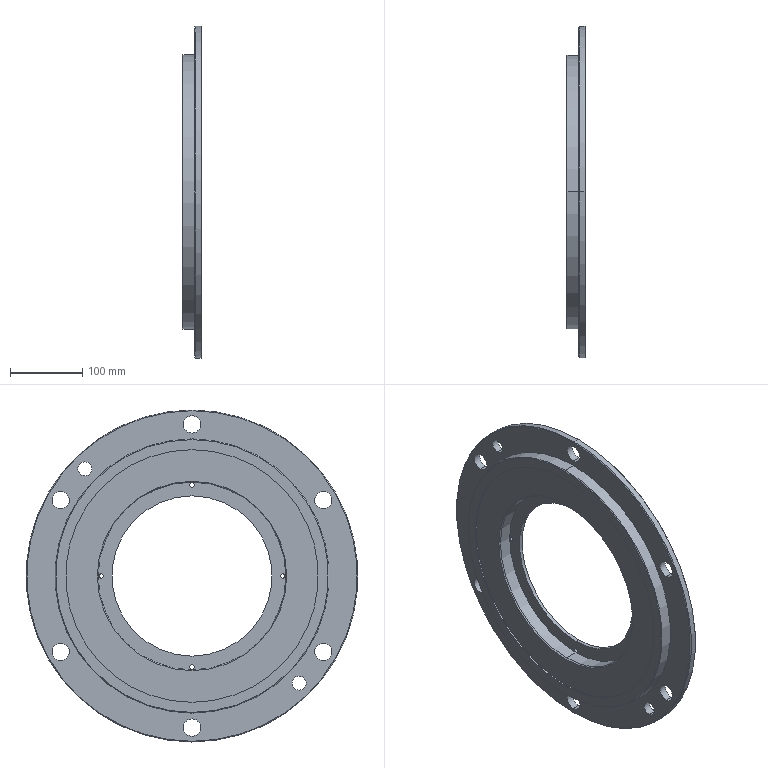Part | SolidWorks | features ICE 4, CirPattern 3, Chamfer 2, 3DProfileFeature 1, HoleWzd 1, Revolution 1 | 1 solid | 47 faces | box 27 x 460 x 460 mm | volume 2105445 mm3 | cylinder 34 | cone 8 | plane 5 | commonest cylinder face diameters 24 x12 6 x8 19.446 x4 222 x2 260 x2 350 x2
STEP:
#1=CARTESIAN_POINT('',(-10.,-148.492,-138.769));
#2=VERTEX_POINT('',#1);
#3=CARTESIAN_POINT('',(-10.,-148.492,-158.216));
#4=VERTEX_POINT('',#3);
#5=CARTESIAN_POINT('',(-10.,-148.492,-148.492));
#6=DIRECTION('',(1.,0.,0.));
#7=DIRECTION('',(0.,0.,-1.));
#8=AXIS2_PLACEMENT_3D('',#5,#6,#7);
#9=CIRCLE('',#8,9.723);
#10=EDGE_CURVE('',#2,#4,#9,.T.);
#11=ORIENTED_EDGE('',*,*,#10,.F.);
#12=CARTESIAN_POINT('',(0.,-148.492,-138.769));
#13=VERTEX_POINT('',#12);
#14=CARTESIAN_POINT('',(0.,-148.492,-138.769));
#15=DIRECTION('',(1.,0.,0.));
#16=VECTOR('',#15,1000.);
#17=LINE('',#14,#16);
#18=EDGE_CURVE('',#2,#13,#17,.T.);
#19=ORIENTED_EDGE('',*,*,#18,.T.);
#20=CARTESIAN_POINT('',(0.,-148.492,-158.216));
#21=VERTEX_POINT('',#20);
#22=CARTESIAN_POINT('',(0.,-148.492,-148.492));
#23=DIRECTION('',(1.,0.,0.));
#24=DIRECTION('',(0.,0.,-1.));
#25=AXIS2_PLACEMENT_3D('',#22,#23,#24);
#26=CIRCLE('',#25,9.723);
#27=EDGE_CURVE('',#13,#21,#26,.T.);
#28=ORIENTED_EDGE('',*,*,#27,.T.);
#29=CARTESIAN_POINT('',(0.,-148.492,-158.216));
#30=DIRECTION('',(1.,0.,0.));
#31=VECTOR('',#30,1000.);
#32=LINE('',#29,#31);
#33=EDGE_CURVE('',#4,#21,#32,.T.);
#34=ORIENTED_EDGE('',*,*,#33,.F.);
#35=EDGE_LOOP('',(#11,#19,#28,#34));
#36=FACE_OUTER_BOUND('',#35,.T.);
#37=CARTESIAN_POINT('',(0.,-148.492,-148.492));
#38=DIRECTION('',(1.,0.,0.));
#39=DIRECTION('',(0.,0.,-1.));
#40=AXIS2_PLACEMENT_3D('',#37,#38,#39);
#41=CYLINDRICAL_SURFACE('',#40,9.723);
#42=ADVANCED_FACE('',(#36),#41,.F.);
#43=CARTESIAN_POINT('',(-10.,148.492,158.216));
#44=VERTEX_POINT('',#43);
#45=CARTESIAN_POINT('',(-10.,148.492,138.769));
#46=VERTEX_POINT('',#45);
#47=CARTESIAN_POINT('',(-10.,148.492,148.492));
#48=DIRECTION('',(1.,0.,0.));
#49=DIRECTION('',(0.,0.,-1.));
#50=AXIS2_PLACEMENT_3D('',#47,#48,#49);
#51=CIRCLE('',#50,9.723);
#52=EDGE_CURVE('',#44,#46,#51,.T.);
#53=ORIENTED_EDGE('',*,*,#52,.F.);
#54=CARTESIAN_POINT('',(0.,148.492,158.216));
#55=VERTEX_POINT('',#54);
#56=CARTESIAN_POINT('',(0.,148.492,158.216));
#57=DIRECTION('',(1.,0.,0.));
#58=VECTOR('',#57,1000.);
#59=LINE('',#56,#58);
#60=EDGE_CURVE('',#44,#55,#59,.T.);
#61=ORIENTED_EDGE('',*,*,#60,.T.);
#62=CARTESIAN_POINT('',(0.,148.492,138.769));
#63=VERTEX_POINT('',#62);
#64=CARTESIAN_POINT('',(0.,148.492,148.492));
#65=DIRECTION('',(1.,0.,0.));
#66=DIRECTION('',(0.,0.,-1.));
#67=AXIS2_PLACEMENT_3D('',#64,#65,#66);
#68=CIRCLE('',#67,9.723);
#69=EDGE_CURVE('',#55,#63,#68,.T.);
#70=ORIENTED_EDGE('',*,*,#69,.T.);
#71=CARTESIAN_POINT('',(0.,148.492,138.769));
#72=DIRECTION('',(1.,0.,0.));
#73=VECTOR('',#72,1000.);
#74=LINE('',#71,#73);
#75=EDGE_CURVE('',#46,#63,#74,.T.);
#76=ORIENTED_EDGE('',*,*,#75,.F.);
#77=EDGE_LOOP('',(#53,#61,#70,#76));
#78=FACE_OUTER_BOUND('',#77,.T.);
#79=CARTESIAN_POINT('',(0.,148.492,148.492));
#80=DIRECTION('',(1.,0.,0.));
#81=DIRECTION('',(0.,0.,-1.));
#82=AXIS2_PLACEMENT_3D('',#79,#80,#81);
#83=CYLINDRICAL_SURFACE('',#82,9.723);
#84=ADVANCED_FACE('',(#78),#83,.F.);
#85=CARTESIAN_POINT('',(-27.,0.,189.));
#86=VERTEX_POINT('',#85);
#87=CARTESIAN_POINT('',(-27.,0.,-189.));
#88=VERTEX_POINT('',#87);
#89=CARTESIAN_POINT('',(-27.,0.,0.));
#90=DIRECTION('',(-1.,0.,0.));
#91=DIRECTION('',(0.,0.,-1.));
#92=AXIS2_PLACEMENT_3D('',#89,#90,#91);
#93=CIRCLE('',#92,189.);
#94=EDGE_CURVE('',#86,#88,#93,.T.);
#95=ORIENTED_EDGE('',*,*,#94,.F.);
#96=CARTESIAN_POINT('',(-26.,0.,190.));
#97=VERTEX_POINT('',#96);
#98=CARTESIAN_POINT('',(-27.,0.,189.));
#99=DIRECTION('',(0.7071,0.,0.7071));
#100=VECTOR('',#99,1000.);
#101=LINE('',#98,#100);
#102=EDGE_CURVE('',#86,#97,#101,.T.);
#103=ORIENTED_EDGE('',*,*,#102,.T.);
#104=CARTESIAN_POINT('',(-26.,0.,-190.));
#105=VERTEX_POINT('',#104);
#106=CARTESIAN_POINT('',(-26.,0.,0.));
#107=DIRECTION('',(1.,0.,0.));
#108=DIRECTION('',(0.,0.,-1.));
#109=AXIS2_PLACEMENT_3D('',#106,#107,#108);
#110=CIRCLE('',#109,190.);
#111=EDGE_CURVE('',#105,#97,#110,.T.);
#112=ORIENTED_EDGE('',*,*,#111,.F.);
#113=CARTESIAN_POINT('',(-27.,0.,-189.));
#114=DIRECTION('',(0.7071,0.,-0.7071));
#115=VECTOR('',#114,1000.);
#116=LINE('',#113,#115);
#117=EDGE_CURVE('',#88,#105,#116,.T.);
#118=ORIENTED_EDGE('',*,*,#117,.F.);
#119=EDGE_LOOP('',(#95,#103,#112,#118));
#120=FACE_OUTER_BOUND('',#119,.T.);
#121=CARTESIAN_POINT('',(-27.,0.,0.));
#122=DIRECTION('',(1.,0.,0.));
#123=DIRECTION('',(0.,0.,-1.));
#124=AXIS2_PLACEMENT_3D('',#121,#122,#123);
#125=CONICAL_SURFACE('',#124,189.,0.7854);
#126=ADVANCED_FACE('',(#120),#125,.T.);
#127=CARTESIAN_POINT('',(-10.,0.,229.));
#128=VERTEX_POINT('',#127);
#129=CARTESIAN_POINT('',(-10.,0.,-229.));
#130=VERTEX_POINT('',#129);
#131=CARTESIAN_POINT('',(-10.,0.,0.));
#132=DIRECTION('',(-1.,0.,0.));
#133=DIRECTION('',(0.,0.,-1.));
#134=AXIS2_PLACEMENT_3D('',#131,#132,#133);
#135=CIRCLE('',#134,229.);
#136=EDGE_CURVE('',#128,#130,#135,.T.);
#137=ORIENTED_EDGE('',*,*,#136,.F.);
#138=CARTESIAN_POINT('',(-9.,0.,230.));
#139=VERTEX_POINT('',#138);
#140=CARTESIAN_POINT('',(-10.,0.,229.));
#141=DIRECTION('',(0.7071,0.,0.7071));
#142=VECTOR('',#141,1000.);
#143=LINE('',#140,#142);
#144=EDGE_CURVE('',#128,#139,#143,.T.);
#145=ORIENTED_EDGE('',*,*,#144,.T.);
#146=CARTESIAN_POINT('',(-9.,0.,-230.));
#147=VERTEX_POINT('',#146);
#148=CARTESIAN_POINT('',(-9.,0.,0.));
#149=DIRECTION('',(1.,0.,0.));
#150=DIRECTION('',(0.,0.,-1.));
#151=AXIS2_PLACEMENT_3D('',#148,#149,#150);
#152=CIRCLE('',#151,230.);
#153=EDGE_CURVE('',#147,#139,#152,.T.);
#154=ORIENTED_EDGE('',*,*,#153,.F.);
#155=CARTESIAN_POINT('',(-10.,0.,-229.));
#156=DIRECTION('',(0.7071,0.,-0.7071));
#157=VECTOR('',#156,1000.);
#158=LINE('',#155,#157);
#159=EDGE_CURVE('',#130,#147,#158,.T.);
#160=ORIENTED_EDGE('',*,*,#159,.F.);
#161=EDGE_LOOP('',(#137,#145,#154,#160));
#162=FACE_OUTER_BOUND('',#161,.T.);
#163=CARTESIAN_POINT('',(-10.,0.,0.));
#164=DIRECTION('',(1.,0.,0.));
#165=DIRECTION('',(0.,0.,-1.));
#166=AXIS2_PLACEMENT_3D('',#163,#164,#165);
#167=CONICAL_SURFACE('',#166,229.,0.7854);
#168=ADVANCED_FACE('',(#162),#167,.T.);
#169=CARTESIAN_POINT('',(0.,0.,-229.));
#170=VERTEX_POINT('',#169);
#171=CARTESIAN_POINT('',(0.,0.,229.));
#172=VERTEX_POINT('',#171);
#173=CARTESIAN_POINT('',(0.,0.,0.));
#174=DIRECTION('',(1.,0.,0.));
#175=DIRECTION('',(0.,0.,1.));
#176=AXIS2_PLACEMENT_3D('',#173,#174,#175);
#177=CIRCLE('',#176,229.);
#178=EDGE_CURVE('',#170,#172,#177,.T.);
#179=ORIENTED_EDGE('',*,*,#178,.F.);
#180=CARTESIAN_POINT('',(-1.,0.,-230.));
#181=VERTEX_POINT('',#180);
#182=CARTESIAN_POINT('',(-1.,0.,-230.));
#183=DIRECTION('',(-0.7071,0.,-0.7071));
#184=VECTOR('',#183,1000.);
#185=LINE('',#182,#184);
#186=EDGE_CURVE('',#170,#181,#185,.T.);
#187=ORIENTED_EDGE('',*,*,#186,.T.);
#188=CARTESIAN_POINT('',(-1.,0.,230.));
#189=VERTEX_POINT('',#188);
#190=CARTESIAN_POINT('',(-1.,0.,0.));
#191=DIRECTION('',(-1.,0.,0.));
#192=DIRECTION('',(0.,0.,1.));
#193=AXIS2_PLACEMENT_3D('',#190,#191,#192);
#194=CIRCLE('',#193,230.);
#195=EDGE_CURVE('',#189,#181,#194,.T.);
#196=ORIENTED_EDGE('',*,*,#195,.F.);
#197=CARTESIAN_POINT('',(-1.,0.,230.));
#198=DIRECTION('',(-0.7071,0.,0.7071));
#199=VECTOR('',#198,1000.);
#200=LINE('',#197,#199);
#201=EDGE_CURVE('',#172,#189,#200,.T.);
#202=ORIENTED_EDGE('',*,*,#201,.F.);
#203=EDGE_LOOP('',(#179,#187,#196,#202));
#204=FACE_OUTER_BOUND('',#203,.T.);
#205=CARTESIAN_POINT('',(-1.,0.,0.));
#206=DIRECTION('',(-1.,0.,0.));
#207=DIRECTION('',(0.,0.,1.));
#208=AXIS2_PLACEMENT_3D('',#205,#206,#207);
#209=CONICAL_SURFACE('',#208,230.,0.7854);
#210=ADVANCED_FACE('',(#204),#209,.T.);
#211=CARTESIAN_POINT('',(-23.,0.,-130.));
#212=VERTEX_POINT('',#211);
#213=CARTESIAN_POINT('',(-23.,0.,130.));
#214=VERTEX_POINT('',#213);
#215=CARTESIAN_POINT('',(-23.,0.,0.));
#216=DIRECTION('',(-1.,0.,0.));
#217=DIRECTION('',(0.,0.,1.));
#218=AXIS2_PLACEMENT_3D('',#215,#216,#217);
#219=CIRCLE('',#218,130.);
#220=EDGE_CURVE('',#212,#214,#219,.T.);
#221=ORIENTED_EDGE('',*,*,#220,.F.);
#222=CARTESIAN_POINT('',(-25.,0.,-131.155));
#223=VERTEX_POINT('',#222);
#224=CARTESIAN_POINT('',(-25.,0.,-131.155));
#225=DIRECTION('',(-0.866,0.,-0.5));
#226=VECTOR('',#225,1000.);
#227=LINE('',#224,#226);
#228=EDGE_CURVE('',#212,#223,#227,.T.);
#229=ORIENTED_EDGE('',*,*,#228,.T.);
#230=CARTESIAN_POINT('',(-25.,0.,131.155));
#231=VERTEX_POINT('',#230);
#232=CARTESIAN_POINT('',(-25.,0.,0.));
#233=DIRECTION('',(1.,0.,0.));
#234=DIRECTION('',(0.,0.,1.));
#235=AXIS2_PLACEMENT_3D('',#232,#233,#234);
#236=CIRCLE('',#235,131.155);
#237=EDGE_CURVE('',#231,#223,#236,.T.);
#238=ORIENTED_EDGE('',*,*,#237,.F.);
#239=CARTESIAN_POINT('',(-25.,0.,131.155));
#240=DIRECTION('',(-0.866,0.,0.5));
#241=VECTOR('',#240,1000.);
#242=LINE('',#239,#241);
#243=EDGE_CURVE('',#214,#231,#242,.T.);
#244=ORIENTED_EDGE('',*,*,#243,.F.);
#245=EDGE_LOOP('',(#221,#229,#238,#244));
#246=FACE_OUTER_BOUND('',#245,.T.);
#247=CARTESIAN_POINT('',(-25.,0.,0.));
#248=DIRECTION('',(-1.,0.,0.));
#249=DIRECTION('',(0.,0.,1.));
#250=AXIS2_PLACEMENT_3D('',#247,#248,#249);
#251=CONICAL_SURFACE('',#250,131.155,0.5236);
#252=ADVANCED_FACE('',(#246),#251,.F.);
#253=CARTESIAN_POINT('',(-25.,0.,-175.));
#254=VERTEX_POINT('',#253);
#255=CARTESIAN_POINT('',(-25.,0.,175.));
#256=VERTEX_POINT('',#255);
#257=CARTESIAN_POINT('',(-25.,0.,0.));
#258=DIRECTION('',(-1.,0.,0.));
#259=DIRECTION('',(0.,0.,1.));
#260=AXIS2_PLACEMENT_3D('',#257,#258,#259);
#261=CIRCLE('',#260,175.);
#262=EDGE_CURVE('',#254,#256,#261,.T.);
#263=ORIENTED_EDGE('',*,*,#262,.F.);
#264=CARTESIAN_POINT('',(-27.,0.,-175.));
#265=VERTEX_POINT('',#264);
#266=CARTESIAN_POINT('',(-25.,0.,-175.));
#267=DIRECTION('',(-1.,0.,0.));
#268=VECTOR('',#267,1000.);
#269=LINE('',#266,#268);
#270=EDGE_CURVE('',#254,#265,#269,.T.);
#271=ORIENTED_EDGE('',*,*,#270,.T.);
#272=CARTESIAN_POINT('',(-27.,0.,175.));
#273=VERTEX_POINT('',#272);
#274=CARTESIAN_POINT('',(-27.,0.,0.));
#275=DIRECTION('',(-1.,0.,0.));
#276=DIRECTION('',(0.,0.,1.));
#277=AXIS2_PLACEMENT_3D('',#274,#275,#276);
#278=CIRCLE('',#277,175.);
#279=EDGE_CURVE('',#265,#273,#278,.T.);
#280=ORIENTED_EDGE('',*,*,#279,.T.);
#281=CARTESIAN_POINT('',(-25.,0.,175.));
#282=DIRECTION('',(-1.,0.,0.));
#283=VECTOR('',#282,1000.);
#284=LINE('',#281,#283);
#285=EDGE_CURVE('',#256,#273,#284,.T.);
#286=ORIENTED_EDGE('',*,*,#285,.F.);
#287=EDGE_LOOP('',(#263,#271,#280,#286));
#288=FACE_OUTER_BOUND('',#287,.T.);
#289=CARTESIAN_POINT('',(-25.,0.,0.));
#290=DIRECTION('',(-1.,0.,0.));
#291=DIRECTION('',(0.,0.,1.));
#292=AXIS2_PLACEMENT_3D('',#289,#290,#291);
#293=CYLINDRICAL_SURFACE('',#292,175.);
#294=ADVANCED_FACE('',(#288),#293,.F.);
#295=CARTESIAN_POINT('',(-10.,-181.865,117.));
#296=VERTEX_POINT('',#295);
#297=CARTESIAN_POINT('',(-10.,-181.865,93.));
#298=VERTEX_POINT('',#297);
#299=CARTESIAN_POINT('',(-10.,-181.865,105.));
#300=DIRECTION('',(1.,0.,0.));
#301=DIRECTION('',(0.,0.,-1.));
#302=AXIS2_PLACEMENT_3D('',#299,#300,#301);
#303=CIRCLE('',#302,12.);
#304=EDGE_CURVE('',#296,#298,#303,.T.);
#305=ORIENTED_EDGE('',*,*,#304,.F.);
#306=CARTESIAN_POINT('',(0.,-181.865,117.));
#307=VERTEX_POINT('',#306);
#308=CARTESIAN_POINT('',(-27.,-181.865,117.));
#309=DIRECTION('',(1.,0.,0.));
#310=VECTOR('',#309,1000.);
#311=LINE('',#308,#310);
#312=EDGE_CURVE('',#296,#307,#311,.T.);
#313=ORIENTED_EDGE('',*,*,#312,.T.);
#314=CARTESIAN_POINT('',(0.,-181.865,93.));
#315=VERTEX_POINT('',#314);
#316=CARTESIAN_POINT('',(0.,-181.865,105.));
#317=DIRECTION('',(1.,0.,0.));
#318=DIRECTION('',(0.,0.866,-0.5));
#319=AXIS2_PLACEMENT_3D('',#316,#317,#318);
#320=CIRCLE('',#319,12.);
#321=EDGE_CURVE('',#307,#315,#320,.T.);
#322=ORIENTED_EDGE('',*,*,#321,.T.);
#323=CARTESIAN_POINT('',(-27.,-181.865,93.));
#324=DIRECTION('',(1.,0.,0.));
#325=VECTOR('',#324,1000.);
#326=LINE('',#323,#325);
#327=EDGE_CURVE('',#298,#315,#326,.T.);
#328=ORIENTED_EDGE('',*,*,#327,.F.);
#329=EDGE_LOOP('',(#305,#313,#322,#328));
#330=FACE_OUTER_BOUND('',#329,.T.);
#331=CARTESIAN_POINT('',(-27.,-181.865,105.));
#332=DIRECTION('',(1.,0.,0.));
#333=DIRECTION('',(0.,0.,-1.));
#334=AXIS2_PLACEMENT_3D('',#331,#332,#333);
#335=CYLINDRICAL_SURFACE('',#334,12.);
#336=ADVANCED_FACE('',(#330),#335,.F.);
#337=CARTESIAN_POINT('',(-10.,-181.865,-93.));
#338=VERTEX_POINT('',#337);
#339=CARTESIAN_POINT('',(-10.,-181.865,-117.));
#340=VERTEX_POINT('',#339);
#341=CARTESIAN_POINT('',(-10.,-181.865,-105.));
#342=DIRECTION('',(1.,0.,0.));
#343=DIRECTION('',(0.,0.,-1.));
#344=AXIS2_PLACEMENT_3D('',#341,#342,#343);
#345=CIRCLE('',#344,12.);
#346=EDGE_CURVE('',#338,#340,#345,.T.);
#347=ORIENTED_EDGE('',*,*,#346,.F.);
#348=CARTESIAN_POINT('',(0.,-181.865,-93.));
#349=VERTEX_POINT('',#348);
#350=CARTESIAN_POINT('',(-27.,-181.865,-93.));
#351=DIRECTION('',(1.,0.,0.));
#352=VECTOR('',#351,1000.);
#353=LINE('',#350,#352);
#354=EDGE_CURVE('',#338,#349,#353,.T.);
#355=ORIENTED_EDGE('',*,*,#354,.T.);
#356=CARTESIAN_POINT('',(0.,-181.865,-117.));
#357=VERTEX_POINT('',#356);
#358=CARTESIAN_POINT('',(0.,-181.865,-105.));
#359=DIRECTION('',(1.,0.,0.));
#360=DIRECTION('',(0.,0.866,0.5));
#361=AXIS2_PLACEMENT_3D('',#358,#359,#360);
#362=CIRCLE('',#361,12.);
#363=EDGE_CURVE('',#349,#357,#362,.T.);
#364=ORIENTED_EDGE('',*,*,#363,.T.);
#365=CARTESIAN_POINT('',(-27.,-181.865,-117.));
#366=DIRECTION('',(1.,0.,0.));
#367=VECTOR('',#366,1000.);
#368=LINE('',#365,#367);
#369=EDGE_CURVE('',#340,#357,#368,.T.);
#370=ORIENTED_EDGE('',*,*,#369,.F.);
#371=EDGE_LOOP('',(#347,#355,#364,#370));
#372=FACE_OUTER_BOUND('',#371,.T.);
#373=CARTESIAN_POINT('',(-27.,-181.865,-105.));
#374=DIRECTION('',(1.,0.,0.));
#375=DIRECTION('',(0.,0.,-1.));
#376=AXIS2_PLACEMENT_3D('',#373,#374,#375);
#377=CYLINDRICAL_SURFACE('',#376,12.);
#378=ADVANCED_FACE('',(#372),#377,.F.);
#379=CARTESIAN_POINT('',(-10.,0.,-198.));
#380=VERTEX_POINT('',#379);
#381=CARTESIAN_POINT('',(-10.,0.,-222.));
#382=VERTEX_POINT('',#381);
#383=CARTESIAN_POINT('',(-10.,0.,-210.));
#384=DIRECTION('',(1.,0.,0.));
#385=DIRECTION('',(0.,0.,-1.));
#386=AXIS2_PLACEMENT_3D('',#383,#384,#385);
#387=CIRCLE('',#386,12.);
#388=EDGE_CURVE('',#380,#382,#387,.T.);
#389=ORIENTED_EDGE('',*,*,#388,.F.);
#390=CARTESIAN_POINT('',(0.,0.,-198.));
#391=VERTEX_POINT('',#390);
#392=CARTESIAN_POINT('',(-27.,0.,-198.));
#393=DIRECTION('',(1.,0.,0.));
#394=VECTOR('',#393,1000.);
#395=LINE('',#392,#394);
#396=EDGE_CURVE('',#380,#391,#395,.T.);
#397=ORIENTED_EDGE('',*,*,#396,.T.);
#398=CARTESIAN_POINT('',(0.,0.,-222.));
#399=VERTEX_POINT('',#398);
#400=CARTESIAN_POINT('',(0.,0.,-210.));
#401=DIRECTION('',(1.,0.,0.));
#402=DIRECTION('',(0.,0.,1.));
#403=AXIS2_PLACEMENT_3D('',#400,#401,#402);
#404=CIRCLE('',#403,12.);
#405=EDGE_CURVE('',#391,#399,#404,.T.);
#406=ORIENTED_EDGE('',*,*,#405,.T.);
#407=CARTESIAN_POINT('',(-27.,0.,-222.));
#408=DIRECTION('',(1.,0.,0.));
#409=VECTOR('',#408,1000.);
#410=LINE('',#407,#409);
#411=EDGE_CURVE('',#382,#399,#410,.T.);
#412=ORIENTED_EDGE('',*,*,#411,.F.);
#413=EDGE_LOOP('',(#389,#397,#406,#412));
#414=FACE_OUTER_BOUND('',#413,.T.);
#415=CARTESIAN_POINT('',(-27.,0.,-210.));
#416=DIRECTION('',(1.,0.,0.));
#417=DIRECTION('',(0.,0.,-1.));
#418=AXIS2_PLACEMENT_3D('',#415,#416,#417);
#419=CYLINDRICAL_SURFACE('',#418,12.);
#420=ADVANCED_FACE('',(#414),#419,.F.);
#421=CARTESIAN_POINT('',(-10.,181.865,-93.));
#422=VERTEX_POINT('',#421);
#423=CARTESIAN_POINT('',(-10.,181.865,-117.));
#424=VERTEX_POINT('',#423);
#425=CARTESIAN_POINT('',(-10.,181.865,-105.));
#426=DIRECTION('',(1.,0.,0.));
#427=DIRECTION('',(0.,0.,-1.));
#428=AXIS2_PLACEMENT_3D('',#425,#426,#427);
#429=CIRCLE('',#428,12.);
#430=EDGE_CURVE('',#422,#424,#429,.T.);
#431=ORIENTED_EDGE('',*,*,#430,.F.);
#432=CARTESIAN_POINT('',(0.,181.865,-93.));
#433=VERTEX_POINT('',#432);
#434=CARTESIAN_POINT('',(-27.,181.865,-93.));
#435=DIRECTION('',(1.,0.,0.));
#436=VECTOR('',#435,1000.);
#437=LINE('',#434,#436);
#438=EDGE_CURVE('',#422,#433,#437,.T.);
#439=ORIENTED_EDGE('',*,*,#438,.T.);
#440=CARTESIAN_POINT('',(0.,181.865,-117.));
#441=VERTEX_POINT('',#440);
#442=CARTESIAN_POINT('',(0.,181.865,-105.));
#443=DIRECTION('',(1.,0.,0.));
#444=DIRECTION('',(0.,-0.866,0.5));
#445=AXIS2_PLACEMENT_3D('',#442,#443,#444);
#446=CIRCLE('',#445,12.);
#447=EDGE_CURVE('',#433,#441,#446,.T.);
#448=ORIENTED_EDGE('',*,*,#447,.T.);
#449=CARTESIAN_POINT('',(-27.,181.865,-117.));
#450=DIRECTION('',(1.,0.,0.));
#451=VECTOR('',#450,1000.);
#452=LINE('',#449,#451);
#453=EDGE_CURVE('',#424,#441,#452,.T.);
#454=ORIENTED_EDGE('',*,*,#453,.F.);
#455=EDGE_LOOP('',(#431,#439,#448,#454));
#456=FACE_OUTER_BOUND('',#455,.T.);
#457=CARTESIAN_POINT('',(-27.,181.865,-105.));
#458=DIRECTION('',(1.,0.,0.));
#459=DIRECTION('',(0.,0.,-1.));
#460=AXIS2_PLACEMENT_3D('',#457,#458,#459);
#461=CYLINDRICAL_SURFACE('',#460,12.);
#462=ADVANCED_FACE('',(#456),#461,.F.);
#463=CARTESIAN_POINT('',(-10.,181.865,117.));
#464=VERTEX_POINT('',#463);
#465=CARTESIAN_POINT('',(-10.,181.865,93.));
#466=VERTEX_POINT('',#465);
#467=CARTESIAN_POINT('',(-10.,181.865,105.));
#468=DIRECTION('',(1.,0.,0.));
#469=DIRECTION('',(0.,0.,-1.));
#470=AXIS2_PLACEMENT_3D('',#467,#468,#469);
#471=CIRCLE('',#470,12.);
#472=EDGE_CURVE('',#464,#466,#471,.T.);
#473=ORIENTED_EDGE('',*,*,#472,.F.);
#474=CARTESIAN_POINT('',(0.,181.865,117.));
#475=VERTEX_POINT('',#474);
#476=CARTESIAN_POINT('',(-27.,181.865,117.));
#477=DIRECTION('',(1.,0.,0.));
#478=VECTOR('',#477,1000.);
#479=LINE('',#476,#478);
#480=EDGE_CURVE('',#464,#475,#479,.T.);
#481=ORIENTED_EDGE('',*,*,#480,.T.);
#482=CARTESIAN_POINT('',(0.,181.865,93.));
#483=VERTEX_POINT('',#482);
#484=CARTESIAN_POINT('',(0.,181.865,105.));
#485=DIRECTION('',(1.,0.,0.));
#486=DIRECTION('',(0.,-0.866,-0.5));
#487=AXIS2_PLACEMENT_3D('',#484,#485,#486);
#488=CIRCLE('',#487,12.);
#489=EDGE_CURVE('',#475,#483,#488,.T.);
#490=ORIENTED_EDGE('',*,*,#489,.T.);
#491=CARTESIAN_POINT('',(-27.,181.865,93.));
#492=DIRECTION('',(1.,0.,0.));
#493=VECTOR('',#492,1000.);
#494=LINE('',#491,#493);
#495=EDGE_CURVE('',#466,#483,#494,.T.);
#496=ORIENTED_EDGE('',*,*,#495,.F.);
#497=EDGE_LOOP('',(#473,#481,#490,#496));
#498=FACE_OUTER_BOUND('',#497,.T.);
#499=CARTESIAN_POINT('',(-27.,181.865,105.));
#500=DIRECTION('',(1.,0.,0.));
#501=DIRECTION('',(0.,0.,-1.));
#502=AXIS2_PLACEMENT_3D('',#499,#500,#501);
#503=CYLINDRICAL_SURFACE('',#502,12.);
#504=ADVANCED_FACE('',(#498),#503,.F.);
#505=CARTESIAN_POINT('',(-10.,0.,222.));
#506=VERTEX_POINT('',#505);
#507=CARTESIAN_POINT('',(-10.,0.,198.));
#508=VERTEX_POINT('',#507);
#509=CARTESIAN_POINT('',(-10.,0.,210.));
#510=DIRECTION('',(1.,0.,0.));
#511=DIRECTION('',(0.,0.,-1.));
#512=AXIS2_PLACEMENT_3D('',#509,#510,#511);
#513=CIRCLE('',#512,12.);
#514=EDGE_CURVE('',#506,#508,#513,.T.);
#515=ORIENTED_EDGE('',*,*,#514,.F.);
#516=CARTESIAN_POINT('',(0.,0.,222.));
#517=VERTEX_POINT('',#516);
#518=CARTESIAN_POINT('',(-27.,0.,222.));
#519=DIRECTION('',(1.,0.,0.));
#520=VECTOR('',#519,1000.);
#521=LINE('',#518,#520);
#522=EDGE_CURVE('',#506,#517,#521,.T.);
#523=ORIENTED_EDGE('',*,*,#522,.T.);
#524=CARTESIAN_POINT('',(0.,0.,198.));
#525=VERTEX_POINT('',#524);
#526=CARTESIAN_POINT('',(0.,0.,210.));
#527=DIRECTION('',(1.,0.,0.));
#528=DIRECTION('',(0.,0.,-1.));
#529=AXIS2_PLACEMENT_3D('',#526,#527,#528);
#530=CIRCLE('',#529,12.);
#531=EDGE_CURVE('',#517,#525,#530,.T.);
#532=ORIENTED_EDGE('',*,*,#531,.T.);
#533=CARTESIAN_POINT('',(-27.,0.,198.));
#534=DIRECTION('',(1.,0.,0.));
#535=VECTOR('',#534,1000.);
#536=LINE('',#533,#535);
#537=EDGE_CURVE('',#508,#525,#536,.T.);
#538=ORIENTED_EDGE('',*,*,#537,.F.);
#539=EDGE_LOOP('',(#515,#523,#532,#538));
#540=FACE_OUTER_BOUND('',#539,.T.);
#541=CARTESIAN_POINT('',(-27.,0.,210.));
#542=DIRECTION('',(1.,0.,0.));
#543=DIRECTION('',(0.,0.,-1.));
#544=AXIS2_PLACEMENT_3D('',#541,#542,#543);
#545=CYLINDRICAL_SURFACE('',#544,12.);
#546=ADVANCED_FACE('',(#540),#545,.F.);
#547=CARTESIAN_POINT('',(-10.,0.,190.));
#548=VERTEX_POINT('',#547);
#549=CARTESIAN_POINT('',(-10.,0.,-190.));
#550=VERTEX_POINT('',#549);
#551=CARTESIAN_POINT('',(-10.,0.,0.));
#552=DIRECTION('',(-1.,0.,0.));
#553=DIRECTION('',(0.,0.,1.));
#554=AXIS2_PLACEMENT_3D('',#551,#552,#553);
#555=CIRCLE('',#554,190.);
#556=EDGE_CURVE('',#548,#550,#555,.T.);
#557=ORIENTED_EDGE('',*,*,#556,.T.);
#558=CARTESIAN_POINT('',(-73.563,0.,-190.));
#559=DIRECTION('',(-1.,0.,0.));
#560=VECTOR('',#559,1000.);
#561=LINE('',#558,#560);
#562=EDGE_CURVE('',#550,#105,#561,.T.);
#563=ORIENTED_EDGE('',*,*,#562,.T.);
#564=ORIENTED_EDGE('',*,*,#111,.T.);
#565=CARTESIAN_POINT('',(-73.563,0.,190.));
#566=DIRECTION('',(-1.,0.,0.));
#567=VECTOR('',#566,1000.);
#568=LINE('',#565,#567);
#569=EDGE_CURVE('',#548,#97,#568,.T.);
#570=ORIENTED_EDGE('',*,*,#569,.F.);
#571=EDGE_LOOP('',(#557,#563,#564,#570));
#572=FACE_OUTER_BOUND('',#571,.T.);
#573=CARTESIAN_POINT('',(-73.563,0.,0.));
#574=DIRECTION('',(-1.,0.,0.));
#575=DIRECTION('',(0.,0.,1.));
#576=AXIS2_PLACEMENT_3D('',#573,#574,#575);
#577=CYLINDRICAL_SURFACE('',#576,190.);
#578=ADVANCED_FACE('',(#572),#577,.T.);
#579=ORIENTED_EDGE('',*,*,#195,.T.);
#580=CARTESIAN_POINT('',(-73.563,0.,-230.));
#581=DIRECTION('',(-1.,0.,0.));
#582=VECTOR('',#581,1000.);
#583=LINE('',#580,#582);
#584=EDGE_CURVE('',#181,#147,#583,.T.);
#585=ORIENTED_EDGE('',*,*,#584,.T.);
#586=ORIENTED_EDGE('',*,*,#153,.T.);
#587=CARTESIAN_POINT('',(-73.563,0.,230.));
#588=DIRECTION('',(-1.,0.,0.));
#589=VECTOR('',#588,1000.);
#590=LINE('',#587,#589);
#591=EDGE_CURVE('',#189,#139,#590,.T.);
#592=ORIENTED_EDGE('',*,*,#591,.F.);
#593=EDGE_LOOP('',(#579,#585,#586,#592));
#594=FACE_OUTER_BOUND('',#593,.T.);
#595=CARTESIAN_POINT('',(-73.563,0.,0.));
#596=DIRECTION('',(-1.,0.,0.));
#597=DIRECTION('',(0.,0.,1.));
#598=AXIS2_PLACEMENT_3D('',#595,#596,#597);
#599=CYLINDRICAL_SURFACE('',#598,230.);
#600=ADVANCED_FACE('',(#594),#599,.T.);
#601=CARTESIAN_POINT('',(-5.,-126.,3.));
#602=VERTEX_POINT('',#601);
#603=CARTESIAN_POINT('',(-5.,-126.,-3.));
#604=VERTEX_POINT('',#603);
#605=CARTESIAN_POINT('',(-5.,-126.,0.));
#606=DIRECTION('',(1.,0.,0.));
#607=DIRECTION('',(0.,0.,1.));
#608=AXIS2_PLACEMENT_3D('',#605,#606,#607);
#609=CIRCLE('',#608,3.);
#610=EDGE_CURVE('',#602,#604,#609,.T.);
#611=ORIENTED_EDGE('',*,*,#610,.F.);
#612=CARTESIAN_POINT('',(0.,-126.,3.));
#613=VERTEX_POINT('',#612);
#614=CARTESIAN_POINT('',(-27.,-126.,3.));
#615=DIRECTION('',(1.,0.,0.));
#616=VECTOR('',#615,1000.);
#617=LINE('',#614,#616);
#618=EDGE_CURVE('',#602,#613,#617,.T.);
#619=ORIENTED_EDGE('',*,*,#618,.T.);
#620=CARTESIAN_POINT('',(0.,-126.,-3.));
#621=VERTEX_POINT('',#620);
#622=CARTESIAN_POINT('',(0.,-126.,0.));
#623=DIRECTION('',(1.,0.,0.));
#624=DIRECTION('',(0.,1.,0.));
#625=AXIS2_PLACEMENT_3D('',#622,#623,#624);
#626=CIRCLE('',#625,3.);
#627=EDGE_CURVE('',#613,#621,#626,.T.);
#628=ORIENTED_EDGE('',*,*,#627,.T.);
#629=CARTESIAN_POINT('',(-27.,-126.,-3.));
#630=DIRECTION('',(1.,0.,0.));
#631=VECTOR('',#630,1000.);
#632=LINE('',#629,#631);
#633=EDGE_CURVE('',#604,#621,#632,.T.);
#634=ORIENTED_EDGE('',*,*,#633,.F.);
#635=EDGE_LOOP('',(#611,#619,#628,#634));
#636=FACE_OUTER_BOUND('',#635,.T.);
#637=CARTESIAN_POINT('',(-27.,-126.,0.));
#638=DIRECTION('',(1.,0.,0.));
#639=DIRECTION('',(0.,0.,-1.));
#640=AXIS2_PLACEMENT_3D('',#637,#638,#639);
#641=CYLINDRICAL_SURFACE('',#640,3.);
#642=ADVANCED_FACE('',(#636),#641,.F.);
#643=CARTESIAN_POINT('',(-5.,0.,-123.));
#644=VERTEX_POINT('',#643);
#645=CARTESIAN_POINT('',(-5.,0.,-129.));
#646=VERTEX_POINT('',#645);
#647=CARTESIAN_POINT('',(-5.,0.,-126.));
#648=DIRECTION('',(1.,0.,0.));
#649=DIRECTION('',(0.,0.,1.));
#650=AXIS2_PLACEMENT_3D('',#647,#648,#649);
#651=CIRCLE('',#650,3.);
#652=EDGE_CURVE('',#644,#646,#651,.T.);
#653=ORIENTED_EDGE('',*,*,#652,.F.);
#654=CARTESIAN_POINT('',(0.,0.,-123.));
#655=VERTEX_POINT('',#654);
#656=CARTESIAN_POINT('',(-27.,0.,-123.));
#657=DIRECTION('',(1.,0.,0.));
#658=VECTOR('',#657,1000.);
#659=LINE('',#656,#658);
#660=EDGE_CURVE('',#644,#655,#659,.T.);
#661=ORIENTED_EDGE('',*,*,#660,.T.);
#662=CARTESIAN_POINT('',(0.,0.,-129.));
#663=VERTEX_POINT('',#662);
#664=CARTESIAN_POINT('',(0.,0.,-126.));
#665=DIRECTION('',(1.,0.,0.));
#666=DIRECTION('',(0.,0.,1.));
#667=AXIS2_PLACEMENT_3D('',#664,#665,#666);
#668=CIRCLE('',#667,3.);
#669=EDGE_CURVE('',#655,#663,#668,.T.);
#670=ORIENTED_EDGE('',*,*,#669,.T.);
#671=CARTESIAN_POINT('',(-27.,0.,-129.));
#672=DIRECTION('',(1.,0.,0.));
#673=VECTOR('',#672,1000.);
#674=LINE('',#671,#673);
#675=EDGE_CURVE('',#646,#663,#674,.T.);
#676=ORIENTED_EDGE('',*,*,#675,.F.);
#677=EDGE_LOOP('',(#653,#661,#670,#676));
#678=FACE_OUTER_BOUND('',#677,.T.);
#679=CARTESIAN_POINT('',(-27.,0.,-126.));
#680=DIRECTION('',(1.,0.,0.));
#681=DIRECTION('',(0.,0.,-1.));
#682=AXIS2_PLACEMENT_3D('',#679,#680,#681);
#683=CYLINDRICAL_SURFACE('',#682,3.);
#684=ADVANCED_FACE('',(#678),#683,.F.);
#685=CARTESIAN_POINT('',(-5.,126.,3.));
#686=VERTEX_POINT('',#685);
#687=CARTESIAN_POINT('',(-5.,126.,-3.));
#688=VERTEX_POINT('',#687);
#689=CARTESIAN_POINT('',(-5.,126.,0.));
#690=DIRECTION('',(1.,0.,0.));
#691=DIRECTION('',(0.,0.,1.));
#692=AXIS2_PLACEMENT_3D('',#689,#690,#691);
#693=CIRCLE('',#692,3.);
#694=EDGE_CURVE('',#686,#688,#693,.T.);
#695=ORIENTED_EDGE('',*,*,#694,.F.);
#696=CARTESIAN_POINT('',(0.,126.,3.));
#697=VERTEX_POINT('',#696);
#698=CARTESIAN_POINT('',(-27.,126.,3.));
#699=DIRECTION('',(1.,0.,0.));
#700=VECTOR('',#699,1000.);
#701=LINE('',#698,#700);
#702=EDGE_CURVE('',#686,#697,#701,.T.);
#703=ORIENTED_EDGE('',*,*,#702,.T.);
#704=CARTESIAN_POINT('',(0.,126.,-3.));
#705=VERTEX_POINT('',#704);
#706=CARTESIAN_POINT('',(0.,126.,0.));
#707=DIRECTION('',(1.,0.,0.));
#708=DIRECTION('',(0.,-1.,0.));
#709=AXIS2_PLACEMENT_3D('',#706,#707,#708);
#710=CIRCLE('',#709,3.);
#711=EDGE_CURVE('',#697,#705,#710,.T.);
#712=ORIENTED_EDGE('',*,*,#711,.T.);
#713=CARTESIAN_POINT('',(-27.,126.,-3.));
#714=DIRECTION('',(1.,0.,0.));
#715=VECTOR('',#714,1000.);
#716=LINE('',#713,#715);
#717=EDGE_CURVE('',#688,#705,#716,.T.);
#718=ORIENTED_EDGE('',*,*,#717,.F.);
#719=EDGE_LOOP('',(#695,#703,#712,#718));
#720=FACE_OUTER_BOUND('',#719,.T.);
#721=CARTESIAN_POINT('',(-27.,126.,0.));
#722=DIRECTION('',(1.,0.,0.));
#723=DIRECTION('',(0.,0.,-1.));
#724=AXIS2_PLACEMENT_3D('',#721,#722,#723);
#725=CYLINDRICAL_SURFACE('',#724,3.);
#726=ADVANCED_FACE('',(#720),#725,.F.);
#727=CARTESIAN_POINT('',(-5.,0.,129.));
#728=VERTEX_POINT('',#727);
#729=CARTESIAN_POINT('',(-5.,0.,123.));
#730=VERTEX_POINT('',#729);
#731=CARTESIAN_POINT('',(-5.,0.,126.));
#732=DIRECTION('',(1.,0.,0.));
#733=DIRECTION('',(0.,0.,1.));
#734=AXIS2_PLACEMENT_3D('',#731,#732,#733);
#735=CIRCLE('',#734,3.);
#736=EDGE_CURVE('',#728,#730,#735,.T.);
#737=ORIENTED_EDGE('',*,*,#736,.F.);
#738=CARTESIAN_POINT('',(0.,0.,129.));
#739=VERTEX_POINT('',#738);
#740=CARTESIAN_POINT('',(-27.,0.,129.));
#741=DIRECTION('',(1.,0.,0.));
#742=VECTOR('',#741,1000.);
#743=LINE('',#740,#742);
#744=EDGE_CURVE('',#728,#739,#743,.T.);
#745=ORIENTED_EDGE('',*,*,#744,.T.);
#746=CARTESIAN_POINT('',(0.,0.,123.));
#747=VERTEX_POINT('',#746);
#748=CARTESIAN_POINT('',(0.,0.,126.));
#749=DIRECTION('',(1.,0.,0.));
#750=DIRECTION('',(0.,0.,-1.));
#751=AXIS2_PLACEMENT_3D('',#748,#749,#750);
#752=CIRCLE('',#751,3.);
#753=EDGE_CURVE('',#739,#747,#752,.T.);
#754=ORIENTED_EDGE('',*,*,#753,.T.);
#755=CARTESIAN_POINT('',(-27.,0.,123.));
#756=DIRECTION('',(1.,0.,0.));
#757=VECTOR('',#756,1000.);
#758=LINE('',#755,#757);
#759=EDGE_CURVE('',#730,#747,#758,.T.);
#760=ORIENTED_EDGE('',*,*,#759,.F.);
#761=EDGE_LOOP('',(#737,#745,#754,#760));
#762=FACE_OUTER_BOUND('',#761,.T.);
#763=CARTESIAN_POINT('',(-27.,0.,126.));
#764=DIRECTION('',(1.,0.,0.));
#765=DIRECTION('',(0.,0.,-1.));
#766=AXIS2_PLACEMENT_3D('',#763,#764,#765);
#767=CYLINDRICAL_SURFACE('',#766,3.);
#768=ADVANCED_FACE('',(#762),#767,.F.);
#769=CARTESIAN_POINT('',(0.,0.,-111.));
#770=VERTEX_POINT('',#769);
#771=CARTESIAN_POINT('',(0.,0.,111.));
#772=VERTEX_POINT('',#771);
#773=CARTESIAN_POINT('',(0.,0.,0.));
#774=DIRECTION('',(-1.,0.,0.));
#775=DIRECTION('',(0.,0.,1.));
#776=AXIS2_PLACEMENT_3D('',#773,#774,#775);
#777=CIRCLE('',#776,111.);
#778=EDGE_CURVE('',#770,#772,#777,.T.);
#779=ORIENTED_EDGE('',*,*,#778,.F.);
#780=CARTESIAN_POINT('',(-5.,0.,-111.));
#781=VERTEX_POINT('',#780);
#782=CARTESIAN_POINT('',(-73.563,0.,-111.));
#783=DIRECTION('',(-1.,0.,0.));
#784=VECTOR('',#783,1000.);
#785=LINE('',#782,#784);
#786=EDGE_CURVE('',#770,#781,#785,.T.);
#787=ORIENTED_EDGE('',*,*,#786,.T.);
#788=CARTESIAN_POINT('',(-5.,0.,111.));
#789=VERTEX_POINT('',#788);
#790=CARTESIAN_POINT('',(-5.,0.,0.));
#791=DIRECTION('',(1.,0.,0.));
#792=DIRECTION('',(0.,0.,1.));
#793=AXIS2_PLACEMENT_3D('',#790,#791,#792);
#794=CIRCLE('',#793,111.);
#795=EDGE_CURVE('',#789,#781,#794,.T.);
#796=ORIENTED_EDGE('',*,*,#795,.F.);
#797=CARTESIAN_POINT('',(-73.563,0.,111.));
#798=DIRECTION('',(-1.,0.,0.));
#799=VECTOR('',#798,1000.);
#800=LINE('',#797,#799);
#801=EDGE_CURVE('',#772,#789,#800,.T.);
#802=ORIENTED_EDGE('',*,*,#801,.F.);
#803=EDGE_LOOP('',(#779,#787,#796,#802));
#804=FACE_OUTER_BOUND('',#803,.T.);
#805=CARTESIAN_POINT('',(-73.563,0.,0.));
#806=DIRECTION('',(-1.,0.,0.));
#807=DIRECTION('',(0.,0.,1.));
#808=AXIS2_PLACEMENT_3D('',#805,#806,#807);
#809=CYLINDRICAL_SURFACE('',#808,111.);
#810=ADVANCED_FACE('',(#804),#809,.F.);
#811=CARTESIAN_POINT('',(-5.,0.,-130.));
#812=VERTEX_POINT('',#811);
#813=CARTESIAN_POINT('',(-5.,0.,130.));
#814=VERTEX_POINT('',#813);
#815=CARTESIAN_POINT('',(-5.,0.,0.));
#816=DIRECTION('',(-1.,0.,0.));
#817=DIRECTION('',(0.,0.,1.));
#818=AXIS2_PLACEMENT_3D('',#815,#816,#817);
#819=CIRCLE('',#818,130.);
#820=EDGE_CURVE('',#812,#814,#819,.T.);
#821=ORIENTED_EDGE('',*,*,#820,.F.);
#822=CARTESIAN_POINT('',(-5.,0.,-130.));
#823=DIRECTION('',(-1.,0.,0.));
#824=VECTOR('',#823,1000.);
#825=LINE('',#822,#824);
#826=EDGE_CURVE('',#812,#212,#825,.T.);
#827=ORIENTED_EDGE('',*,*,#826,.T.);
#828=ORIENTED_EDGE('',*,*,#220,.T.);
#829=CARTESIAN_POINT('',(-5.,0.,130.));
#830=DIRECTION('',(-1.,0.,0.));
#831=VECTOR('',#830,1000.);
#832=LINE('',#829,#831);
#833=EDGE_CURVE('',#814,#214,#832,.T.);
#834=ORIENTED_EDGE('',*,*,#833,.F.);
#835=EDGE_LOOP('',(#821,#827,#828,#834));
#836=FACE_OUTER_BOUND('',#835,.T.);
#837=CARTESIAN_POINT('',(-5.,0.,0.));
#838=DIRECTION('',(-1.,0.,0.));
#839=DIRECTION('',(0.,0.,1.));
#840=AXIS2_PLACEMENT_3D('',#837,#838,#839);
#841=CYLINDRICAL_SURFACE('',#840,130.);
#842=ADVANCED_FACE('',(#836),#841,.F.);
#843=CARTESIAN_POINT('',(0.,148.492,148.492));
#844=DIRECTION('',(1.,0.,0.));
#845=DIRECTION('',(0.,0.,-1.));
#846=AXIS2_PLACEMENT_3D('',#843,#844,#845);
#847=CIRCLE('',#846,9.723);
#848=EDGE_CURVE('',#63,#55,#847,.T.);
#849=ORIENTED_EDGE('',*,*,#848,.F.);
#850=ORIENTED_EDGE('',*,*,#69,.F.);
#851=EDGE_LOOP('',(#849,#850));
#852=FACE_BOUND('',#851,.T.);
#853=CARTESIAN_POINT('',(0.,0.,0.));
#854=DIRECTION('',(1.,0.,0.));
#855=DIRECTION('',(0.,0.,1.));
#856=AXIS2_PLACEMENT_3D('',#853,#854,#855);
#857=CIRCLE('',#856,229.);
#858=EDGE_CURVE('',#172,#170,#857,.T.);
#859=ORIENTED_EDGE('',*,*,#858,.T.);
#860=ORIENTED_EDGE('',*,*,#178,.T.);
#861=EDGE_LOOP('',(#859,#860));
#862=FACE_OUTER_BOUND('',#861,.T.);
#863=CARTESIAN_POINT('',(0.,-126.,0.));
#864=DIRECTION('',(1.,0.,0.));
#865=DIRECTION('',(0.,1.,0.));
#866=AXIS2_PLACEMENT_3D('',#863,#864,#865);
#867=CIRCLE('',#866,3.);
#868=EDGE_CURVE('',#621,#613,#867,.T.);
#869=ORIENTED_EDGE('',*,*,#868,.F.);
#870=ORIENTED_EDGE('',*,*,#627,.F.);
#871=EDGE_LOOP('',(#869,#870));
#872=FACE_BOUND('',#871,.T.);
#873=CARTESIAN_POINT('',(0.,0.,-126.));
#874=DIRECTION('',(1.,0.,0.));
#875=DIRECTION('',(0.,0.,1.));
#876=AXIS2_PLACEMENT_3D('',#873,#874,#875);
#877=CIRCLE('',#876,3.);
#878=EDGE_CURVE('',#663,#655,#877,.T.);
#879=ORIENTED_EDGE('',*,*,#878,.F.);
#880=ORIENTED_EDGE('',*,*,#669,.F.);
#881=EDGE_LOOP('',(#879,#880));
#882=FACE_BOUND('',#881,.T.);
#883=CARTESIAN_POINT('',(0.,126.,0.));
#884=DIRECTION('',(1.,0.,0.));
#885=DIRECTION('',(0.,-1.,0.));
#886=AXIS2_PLACEMENT_3D('',#883,#884,#885);
#887=CIRCLE('',#886,3.);
#888=EDGE_CURVE('',#705,#697,#887,.T.);
#889=ORIENTED_EDGE('',*,*,#888,.F.);
#890=ORIENTED_EDGE('',*,*,#711,.F.);
#891=EDGE_LOOP('',(#889,#890));
#892=FACE_BOUND('',#891,.T.);
#893=CARTESIAN_POINT('',(0.,0.,126.));
#894=DIRECTION('',(1.,0.,0.));
#895=DIRECTION('',(0.,0.,-1.));
#896=AXIS2_PLACEMENT_3D('',#893,#894,#895);
#897=CIRCLE('',#896,3.);
#898=EDGE_CURVE('',#747,#739,#897,.T.);
#899=ORIENTED_EDGE('',*,*,#898,.F.);
#900=ORIENTED_EDGE('',*,*,#753,.F.);
#901=EDGE_LOOP('',(#899,#900));
#902=FACE_BOUND('',#901,.T.);
#903=CARTESIAN_POINT('',(0.,-181.865,105.));
#904=DIRECTION('',(1.,0.,0.));
#905=DIRECTION('',(0.,0.866,-0.5));
#906=AXIS2_PLACEMENT_3D('',#903,#904,#905);
#907=CIRCLE('',#906,12.);
#908=EDGE_CURVE('',#315,#307,#907,.T.);
#909=ORIENTED_EDGE('',*,*,#908,.F.);
#910=ORIENTED_EDGE('',*,*,#321,.F.);
#911=EDGE_LOOP('',(#909,#910));
#912=FACE_BOUND('',#911,.T.);
#913=CARTESIAN_POINT('',(0.,-181.865,-105.));
#914=DIRECTION('',(1.,0.,0.));
#915=DIRECTION('',(0.,0.866,0.5));
#916=AXIS2_PLACEMENT_3D('',#913,#914,#915);
#917=CIRCLE('',#916,12.);
#918=EDGE_CURVE('',#357,#349,#917,.T.);
#919=ORIENTED_EDGE('',*,*,#918,.F.);
#920=ORIENTED_EDGE('',*,*,#363,.F.);
#921=EDGE_LOOP('',(#919,#920));
#922=FACE_BOUND('',#921,.T.);
#923=CARTESIAN_POINT('',(0.,0.,-210.));
#924=DIRECTION('',(1.,0.,0.));
#925=DIRECTION('',(0.,0.,1.));
#926=AXIS2_PLACEMENT_3D('',#923,#924,#925);
#927=CIRCLE('',#926,12.);
#928=EDGE_CURVE('',#399,#391,#927,.T.);
#929=ORIENTED_EDGE('',*,*,#928,.F.);
#930=ORIENTED_EDGE('',*,*,#405,.F.);
#931=EDGE_LOOP('',(#929,#930));
#932=FACE_BOUND('',#931,.T.);
#933=CARTESIAN_POINT('',(0.,181.865,-105.));
#934=DIRECTION('',(1.,0.,0.));
#935=DIRECTION('',(0.,-0.866,0.5));
#936=AXIS2_PLACEMENT_3D('',#933,#934,#935);
#937=CIRCLE('',#936,12.);
#938=EDGE_CURVE('',#441,#433,#937,.T.);
#939=ORIENTED_EDGE('',*,*,#938,.F.);
#940=ORIENTED_EDGE('',*,*,#447,.F.);
#941=EDGE_LOOP('',(#939,#940));
#942=FACE_BOUND('',#941,.T.);
#943=CARTESIAN_POINT('',(0.,181.865,105.));
#944=DIRECTION('',(1.,0.,0.));
#945=DIRECTION('',(0.,-0.866,-0.5));
#946=AXIS2_PLACEMENT_3D('',#943,#944,#945);
#947=CIRCLE('',#946,12.);
#948=EDGE_CURVE('',#483,#475,#947,.T.);
#949=ORIENTED_EDGE('',*,*,#948,.F.);
#950=ORIENTED_EDGE('',*,*,#489,.F.);
#951=EDGE_LOOP('',(#949,#950));
#952=FACE_BOUND('',#951,.T.);
#953=CARTESIAN_POINT('',(0.,0.,210.));
#954=DIRECTION('',(1.,0.,0.));
#955=DIRECTION('',(0.,0.,-1.));
#956=AXIS2_PLACEMENT_3D('',#953,#954,#955);
#957=CIRCLE('',#956,12.);
#958=EDGE_CURVE('',#525,#517,#957,.T.);
#959=ORIENTED_EDGE('',*,*,#958,.F.);
#960=ORIENTED_EDGE('',*,*,#531,.F.);
#961=EDGE_LOOP('',(#959,#960));
#962=FACE_BOUND('',#961,.T.);
#963=CARTESIAN_POINT('',(0.,0.,0.));
#964=DIRECTION('',(-1.,0.,0.));
#965=DIRECTION('',(0.,0.,1.));
#966=AXIS2_PLACEMENT_3D('',#963,#964,#965);
#967=CIRCLE('',#966,111.);
#968=EDGE_CURVE('',#772,#770,#967,.T.);
#969=ORIENTED_EDGE('',*,*,#968,.T.);
#970=ORIENTED_EDGE('',*,*,#778,.T.);
#971=EDGE_LOOP('',(#969,#970));
#972=FACE_BOUND('',#971,.T.);
#973=CARTESIAN_POINT('',(0.,-148.492,-148.492));
#974=DIRECTION('',(1.,0.,0.));
#975=DIRECTION('',(0.,0.,-1.));
#976=AXIS2_PLACEMENT_3D('',#973,#974,#975);
#977=CIRCLE('',#976,9.723);
#978=EDGE_CURVE('',#21,#13,#977,.T.);
#979=ORIENTED_EDGE('',*,*,#978,.F.);
#980=ORIENTED_EDGE('',*,*,#27,.F.);
#981=EDGE_LOOP('',(#979,#980));
#982=FACE_BOUND('',#981,.T.);
#983=CARTESIAN_POINT('',(0.,111.,0.));
#984=DIRECTION('',(-1.,0.,0.));
#985=DIRECTION('',(0.,0.,1.));
#986=AXIS2_PLACEMENT_3D('',#983,#984,#985);
#987=PLANE('',#986);
#988=ADVANCED_FACE('',(#852,#862,#872,#882,#892,#902,#912,#922,#932,#942,#952,#962,#972,#982),#987,.F.);
#989=ORIENTED_EDGE('',*,*,#826,.F.);
#990=CARTESIAN_POINT('',(-5.,0.,0.));
#991=DIRECTION('',(-1.,0.,0.));
#992=DIRECTION('',(0.,0.,1.));
#993=AXIS2_PLACEMENT_3D('',#990,#991,#992);
#994=CIRCLE('',#993,130.);
#995=EDGE_CURVE('',#814,#812,#994,.T.);
#996=ORIENTED_EDGE('',*,*,#995,.F.);
#997=ORIENTED_EDGE('',*,*,#833,.T.);
#998=CARTESIAN_POINT('',(-23.,0.,0.));
#999=DIRECTION('',(-1.,0.,0.));
#1000=DIRECTION('',(0.,0.,1.));
#1001=AXIS2_PLACEMENT_3D('',#998,#999,#1000);
#1002=CIRCLE('',#1001,130.);
#1003=EDGE_CURVE('',#214,#212,#1002,.T.);
#1004=ORIENTED_EDGE('',*,*,#1003,.T.);
#1005=EDGE_LOOP('',(#989,#996,#997,#1004));
#1006=FACE_OUTER_BOUND('',#1005,.T.);
#1007=CARTESIAN_POINT('',(-5.,0.,0.));
#1008=DIRECTION('',(-1.,0.,0.));
#1009=DIRECTION('',(0.,0.,1.));
#1010=AXIS2_PLACEMENT_3D('',#1007,#1008,#1009);
#1011=CYLINDRICAL_SURFACE('',#1010,130.);
#1012=ADVANCED_FACE('',(#1006),#1011,.F.);
#1013=ORIENTED_EDGE('',*,*,#786,.F.);
#1014=ORIENTED_EDGE('',*,*,#968,.F.);
#1015=ORIENTED_EDGE('',*,*,#801,.T.);
#1016=CARTESIAN_POINT('',(-5.,0.,0.));
#1017=DIRECTION('',(1.,0.,0.));
#1018=DIRECTION('',(0.,0.,1.));
#1019=AXIS2_PLACEMENT_3D('',#1016,#1017,#1018);
#1020=CIRCLE('',#1019,111.);
#1021=EDGE_CURVE('',#781,#789,#1020,.T.);
#1022=ORIENTED_EDGE('',*,*,#1021,.F.);
#1023=EDGE_LOOP('',(#1013,#1014,#1015,#1022));
#1024=FACE_OUTER_BOUND('',#1023,.T.);
#1025=CARTESIAN_POINT('',(-73.563,0.,0.));
#1026=DIRECTION('',(-1.,0.,0.));
#1027=DIRECTION('',(0.,0.,1.));
#1028=AXIS2_PLACEMENT_3D('',#1025,#1026,#1027);
#1029=CYLINDRICAL_SURFACE('',#1028,111.);
#1030=ADVANCED_FACE('',(#1024),#1029,.F.);
#1031=ORIENTED_EDGE('',*,*,#744,.F.);
#1032=CARTESIAN_POINT('',(-5.,0.,126.));
#1033=DIRECTION('',(1.,0.,0.));
#1034=DIRECTION('',(0.,0.,1.));
#1035=AXIS2_PLACEMENT_3D('',#1032,#1033,#1034);
#1036=CIRCLE('',#1035,3.);
#1037=EDGE_CURVE('',#730,#728,#1036,.T.);
#1038=ORIENTED_EDGE('',*,*,#1037,.F.);
#1039=ORIENTED_EDGE('',*,*,#759,.T.);
#1040=ORIENTED_EDGE('',*,*,#898,.T.);
#1041=EDGE_LOOP('',(#1031,#1038,#1039,#1040));
#1042=FACE_OUTER_BOUND('',#1041,.T.);
#1043=CARTESIAN_POINT('',(-27.,0.,126.));
#1044=DIRECTION('',(1.,0.,0.));
#1045=DIRECTION('',(0.,0.,-1.));
#1046=AXIS2_PLACEMENT_3D('',#1043,#1044,#1045);
#1047=CYLINDRICAL_SURFACE('',#1046,3.);
#1048=ADVANCED_FACE('',(#1042),#1047,.F.);
#1049=ORIENTED_EDGE('',*,*,#702,.F.);
#1050=CARTESIAN_POINT('',(-5.,126.,0.));
#1051=DIRECTION('',(1.,0.,0.));
#1052=DIRECTION('',(0.,0.,1.));
#1053=AXIS2_PLACEMENT_3D('',#1050,#1051,#1052);
#1054=CIRCLE('',#1053,3.);
#1055=EDGE_CURVE('',#688,#686,#1054,.T.);
#1056=ORIENTED_EDGE('',*,*,#1055,.F.);
#1057=ORIENTED_EDGE('',*,*,#717,.T.);
#1058=ORIENTED_EDGE('',*,*,#888,.T.);
#1059=EDGE_LOOP('',(#1049,#1056,#1057,#1058));
#1060=FACE_OUTER_BOUND('',#1059,.T.);
#1061=CARTESIAN_POINT('',(-27.,126.,0.));
#1062=DIRECTION('',(1.,0.,0.));
#1063=DIRECTION('',(0.,0.,-1.));
#1064=AXIS2_PLACEMENT_3D('',#1061,#1062,#1063);
#1065=CYLINDRICAL_SURFACE('',#1064,3.);
#1066=ADVANCED_FACE('',(#1060),#1065,.F.);
#1067=ORIENTED_EDGE('',*,*,#660,.F.);
#1068=CARTESIAN_POINT('',(-5.,0.,-126.));
#1069=DIRECTION('',(1.,0.,0.));
#1070=DIRECTION('',(0.,0.,1.));
#1071=AXIS2_PLACEMENT_3D('',#1068,#1069,#1070);
#1072=CIRCLE('',#1071,3.);
#1073=EDGE_CURVE('',#646,#644,#1072,.T.);
#1074=ORIENTED_EDGE('',*,*,#1073,.F.);
#1075=ORIENTED_EDGE('',*,*,#675,.T.);
#1076=ORIENTED_EDGE('',*,*,#878,.T.);
#1077=EDGE_LOOP('',(#1067,#1074,#1075,#1076));
#1078=FACE_OUTER_BOUND('',#1077,.T.);
#1079=CARTESIAN_POINT('',(-27.,0.,-126.));
#1080=DIRECTION('',(1.,0.,0.));
#1081=DIRECTION('',(0.,0.,-1.));
#1082=AXIS2_PLACEMENT_3D('',#1079,#1080,#1081);
#1083=CYLINDRICAL_SURFACE('',#1082,3.);
#1084=ADVANCED_FACE('',(#1078),#1083,.F.);
#1085=ORIENTED_EDGE('',*,*,#618,.F.);
#1086=CARTESIAN_POINT('',(-5.,-126.,0.));
#1087=DIRECTION('',(1.,0.,0.));
#1088=DIRECTION('',(0.,0.,1.));
#1089=AXIS2_PLACEMENT_3D('',#1086,#1087,#1088);
#1090=CIRCLE('',#1089,3.);
#1091=EDGE_CURVE('',#604,#602,#1090,.T.);
#1092=ORIENTED_EDGE('',*,*,#1091,.F.);
#1093=ORIENTED_EDGE('',*,*,#633,.T.);
#1094=ORIENTED_EDGE('',*,*,#868,.T.);
#1095=EDGE_LOOP('',(#1085,#1092,#1093,#1094));
#1096=FACE_OUTER_BOUND('',#1095,.T.);
#1097=CARTESIAN_POINT('',(-27.,-126.,0.));
#1098=DIRECTION('',(1.,0.,0.));
#1099=DIRECTION('',(0.,0.,-1.));
#1100=AXIS2_PLACEMENT_3D('',#1097,#1098,#1099);
#1101=CYLINDRICAL_SURFACE('',#1100,3.);
#1102=ADVANCED_FACE('',(#1096),#1101,.F.);
#1103=ORIENTED_EDGE('',*,*,#584,.F.);
#1104=CARTESIAN_POINT('',(-1.,0.,0.));
#1105=DIRECTION('',(-1.,0.,0.));
#1106=DIRECTION('',(0.,0.,1.));
#1107=AXIS2_PLACEMENT_3D('',#1104,#1105,#1106);
#1108=CIRCLE('',#1107,230.);
#1109=EDGE_CURVE('',#181,#189,#1108,.T.);
#1110=ORIENTED_EDGE('',*,*,#1109,.T.);
#1111=ORIENTED_EDGE('',*,*,#591,.T.);
#1112=CARTESIAN_POINT('',(-9.,0.,0.));
#1113=DIRECTION('',(1.,0.,0.));
#1114=DIRECTION('',(0.,0.,-1.));
#1115=AXIS2_PLACEMENT_3D('',#1112,#1113,#1114);
#1116=CIRCLE('',#1115,230.);
#1117=EDGE_CURVE('',#139,#147,#1116,.T.);
#1118=ORIENTED_EDGE('',*,*,#1117,.T.);
#1119=EDGE_LOOP('',(#1103,#1110,#1111,#1118));
#1120=FACE_OUTER_BOUND('',#1119,.T.);
#1121=CARTESIAN_POINT('',(-73.563,0.,0.));
#1122=DIRECTION('',(-1.,0.,0.));
#1123=DIRECTION('',(0.,0.,1.));
#1124=AXIS2_PLACEMENT_3D('',#1121,#1122,#1123);
#1125=CYLINDRICAL_SURFACE('',#1124,230.);
#1126=ADVANCED_FACE('',(#1120),#1125,.T.);
#1127=CARTESIAN_POINT('',(-10.,-148.492,-148.492));
#1128=DIRECTION('',(1.,0.,0.));
#1129=DIRECTION('',(0.,0.,-1.));
#1130=AXIS2_PLACEMENT_3D('',#1127,#1128,#1129);
#1131=CIRCLE('',#1130,9.723);
#1132=EDGE_CURVE('',#4,#2,#1131,.T.);
#1133=ORIENTED_EDGE('',*,*,#1132,.T.);
#1134=ORIENTED_EDGE('',*,*,#10,.T.);
#1135=EDGE_LOOP('',(#1133,#1134));
#1136=FACE_BOUND('',#1135,.T.);
#1137=CARTESIAN_POINT('',(-10.,148.492,148.492));
#1138=DIRECTION('',(1.,0.,0.));
#1139=DIRECTION('',(0.,0.,-1.));
#1140=AXIS2_PLACEMENT_3D('',#1137,#1138,#1139);
#1141=CIRCLE('',#1140,9.723);
#1142=EDGE_CURVE('',#46,#44,#1141,.T.);
#1143=ORIENTED_EDGE('',*,*,#1142,.T.);
#1144=ORIENTED_EDGE('',*,*,#52,.T.);
#1145=EDGE_LOOP('',(#1143,#1144));
#1146=FACE_BOUND('',#1145,.T.);
#1147=CARTESIAN_POINT('',(-10.,0.,0.));
#1148=DIRECTION('',(-1.,0.,0.));
#1149=DIRECTION('',(0.,0.,-1.));
#1150=AXIS2_PLACEMENT_3D('',#1147,#1148,#1149);
#1151=CIRCLE('',#1150,229.);
#1152=EDGE_CURVE('',#130,#128,#1151,.T.);
#1153=ORIENTED_EDGE('',*,*,#1152,.T.);
#1154=ORIENTED_EDGE('',*,*,#136,.T.);
#1155=EDGE_LOOP('',(#1153,#1154));
#1156=FACE_OUTER_BOUND('',#1155,.T.);
#1157=CARTESIAN_POINT('',(-10.,-181.865,105.));
#1158=DIRECTION('',(1.,0.,0.));
#1159=DIRECTION('',(0.,0.,-1.));
#1160=AXIS2_PLACEMENT_3D('',#1157,#1158,#1159);
#1161=CIRCLE('',#1160,12.);
#1162=EDGE_CURVE('',#298,#296,#1161,.T.);
#1163=ORIENTED_EDGE('',*,*,#1162,.T.);
#1164=ORIENTED_EDGE('',*,*,#304,.T.);
#1165=EDGE_LOOP('',(#1163,#1164));
#1166=FACE_BOUND('',#1165,.T.);
#1167=CARTESIAN_POINT('',(-10.,-181.865,-105.));
#1168=DIRECTION('',(1.,0.,0.));
#1169=DIRECTION('',(0.,0.,-1.));
#1170=AXIS2_PLACEMENT_3D('',#1167,#1168,#1169);
#1171=CIRCLE('',#1170,12.);
#1172=EDGE_CURVE('',#340,#338,#1171,.T.);
#1173=ORIENTED_EDGE('',*,*,#1172,.T.);
#1174=ORIENTED_EDGE('',*,*,#346,.T.);
#1175=EDGE_LOOP('',(#1173,#1174));
#1176=FACE_BOUND('',#1175,.T.);
#1177=CARTESIAN_POINT('',(-10.,0.,-210.));
#1178=DIRECTION('',(1.,0.,0.));
#1179=DIRECTION('',(0.,0.,-1.));
#1180=AXIS2_PLACEMENT_3D('',#1177,#1178,#1179);
#1181=CIRCLE('',#1180,12.);
#1182=EDGE_CURVE('',#382,#380,#1181,.T.);
#1183=ORIENTED_EDGE('',*,*,#1182,.T.);
#1184=ORIENTED_EDGE('',*,*,#388,.T.);
#1185=EDGE_LOOP('',(#1183,#1184));
#1186=FACE_BOUND('',#1185,.T.);
#1187=CARTESIAN_POINT('',(-10.,181.865,-105.));
#1188=DIRECTION('',(1.,0.,0.));
#1189=DIRECTION('',(0.,0.,-1.));
#1190=AXIS2_PLACEMENT_3D('',#1187,#1188,#1189);
#1191=CIRCLE('',#1190,12.);
#1192=EDGE_CURVE('',#424,#422,#1191,.T.);
#1193=ORIENTED_EDGE('',*,*,#1192,.T.);
#1194=ORIENTED_EDGE('',*,*,#430,.T.);
#1195=EDGE_LOOP('',(#1193,#1194));
#1196=FACE_BOUND('',#1195,.T.);
#1197=CARTESIAN_POINT('',(-10.,181.865,105.));
#1198=DIRECTION('',(1.,0.,0.));
#1199=DIRECTION('',(0.,0.,-1.));
#1200=AXIS2_PLACEMENT_3D('',#1197,#1198,#1199);
#1201=CIRCLE('',#1200,12.);
#1202=EDGE_CURVE('',#466,#464,#1201,.T.);
#1203=ORIENTED_EDGE('',*,*,#1202,.T.);
#1204=ORIENTED_EDGE('',*,*,#472,.T.);
#1205=EDGE_LOOP('',(#1203,#1204));
#1206=FACE_BOUND('',#1205,.T.);
#1207=CARTESIAN_POINT('',(-10.,0.,210.));
#1208=DIRECTION('',(1.,0.,0.));
#1209=DIRECTION('',(0.,0.,-1.));
#1210=AXIS2_PLACEMENT_3D('',#1207,#1208,#1209);
#1211=CIRCLE('',#1210,12.);
#1212=EDGE_CURVE('',#508,#506,#1211,.T.);
#1213=ORIENTED_EDGE('',*,*,#1212,.T.);
#1214=ORIENTED_EDGE('',*,*,#514,.T.);
#1215=EDGE_LOOP('',(#1213,#1214));
#1216=FACE_BOUND('',#1215,.T.);
#1217=ORIENTED_EDGE('',*,*,#556,.F.);
#1218=CARTESIAN_POINT('',(-10.,0.,0.));
#1219=DIRECTION('',(-1.,0.,0.));
#1220=DIRECTION('',(0.,0.,1.));
#1221=AXIS2_PLACEMENT_3D('',#1218,#1219,#1220);
#1222=CIRCLE('',#1221,190.);
#1223=EDGE_CURVE('',#550,#548,#1222,.T.);
#1224=ORIENTED_EDGE('',*,*,#1223,.F.);
#1225=EDGE_LOOP('',(#1217,#1224));
#1226=FACE_BOUND('',#1225,.T.);
#1227=CARTESIAN_POINT('',(-10.,230.,0.));
#1228=DIRECTION('',(1.,0.,0.));
#1229=DIRECTION('',(0.,0.,-1.));
#1230=AXIS2_PLACEMENT_3D('',#1227,#1228,#1229);
#1231=PLANE('',#1230);
#1232=ADVANCED_FACE('',(#1136,#1146,#1156,#1166,#1176,#1186,#1196,#1206,#1216,#1226),#1231,.F.);
#1233=ORIENTED_EDGE('',*,*,#562,.F.);
#1234=ORIENTED_EDGE('',*,*,#1223,.T.);
#1235=ORIENTED_EDGE('',*,*,#569,.T.);
#1236=CARTESIAN_POINT('',(-26.,0.,0.));
#1237=DIRECTION('',(1.,0.,0.));
#1238=DIRECTION('',(0.,0.,-1.));
#1239=AXIS2_PLACEMENT_3D('',#1236,#1237,#1238);
#1240=CIRCLE('',#1239,190.);
#1241=EDGE_CURVE('',#97,#105,#1240,.T.);
#1242=ORIENTED_EDGE('',*,*,#1241,.T.);
#1243=EDGE_LOOP('',(#1233,#1234,#1235,#1242));
#1244=FACE_OUTER_BOUND('',#1243,.T.);
#1245=CARTESIAN_POINT('',(-73.563,0.,0.));
#1246=DIRECTION('',(-1.,0.,0.));
#1247=DIRECTION('',(0.,0.,1.));
#1248=AXIS2_PLACEMENT_3D('',#1245,#1246,#1247);
#1249=CYLINDRICAL_SURFACE('',#1248,190.);
#1250=ADVANCED_FACE('',(#1244),#1249,.T.);
#1251=CARTESIAN_POINT('',(-27.,0.,0.));
#1252=DIRECTION('',(-1.,0.,0.));
#1253=DIRECTION('',(0.,0.,-1.));
#1254=AXIS2_PLACEMENT_3D('',#1251,#1252,#1253);
#1255=CIRCLE('',#1254,189.);
#1256=EDGE_CURVE('',#88,#86,#1255,.T.);
#1257=ORIENTED_EDGE('',*,*,#1256,.T.);
#1258=ORIENTED_EDGE('',*,*,#94,.T.);
#1259=EDGE_LOOP('',(#1257,#1258));
#1260=FACE_OUTER_BOUND('',#1259,.T.);
#1261=CARTESIAN_POINT('',(-27.,0.,0.));
#1262=DIRECTION('',(-1.,0.,0.));
#1263=DIRECTION('',(0.,0.,1.));
#1264=AXIS2_PLACEMENT_3D('',#1261,#1262,#1263);
#1265=CIRCLE('',#1264,175.);
#1266=EDGE_CURVE('',#273,#265,#1265,.T.);
#1267=ORIENTED_EDGE('',*,*,#1266,.F.);
#1268=ORIENTED_EDGE('',*,*,#279,.F.);
#1269=EDGE_LOOP('',(#1267,#1268));
#1270=FACE_BOUND('',#1269,.T.);
#1271=CARTESIAN_POINT('',(-27.,190.,0.));
#1272=DIRECTION('',(1.,0.,0.));
#1273=DIRECTION('',(0.,0.,-1.));
#1274=AXIS2_PLACEMENT_3D('',#1271,#1272,#1273);
#1275=PLANE('',#1274);
#1276=ADVANCED_FACE('',(#1260,#1270),#1275,.F.);
#1277=ORIENTED_EDGE('',*,*,#522,.F.);
#1278=ORIENTED_EDGE('',*,*,#1212,.F.);
#1279=ORIENTED_EDGE('',*,*,#537,.T.);
#1280=ORIENTED_EDGE('',*,*,#958,.T.);
#1281=EDGE_LOOP('',(#1277,#1278,#1279,#1280));
#1282=FACE_OUTER_BOUND('',#1281,.T.);
#1283=CARTESIAN_POINT('',(-27.,0.,210.));
#1284=DIRECTION('',(1.,0.,0.));
#1285=DIRECTION('',(0.,0.,-1.));
#1286=AXIS2_PLACEMENT_3D('',#1283,#1284,#1285);
#1287=CYLINDRICAL_SURFACE('',#1286,12.);
#1288=ADVANCED_FACE('',(#1282),#1287,.F.);
#1289=ORIENTED_EDGE('',*,*,#480,.F.);
#1290=ORIENTED_EDGE('',*,*,#1202,.F.);
#1291=ORIENTED_EDGE('',*,*,#495,.T.);
#1292=ORIENTED_EDGE('',*,*,#948,.T.);
#1293=EDGE_LOOP('',(#1289,#1290,#1291,#1292));
#1294=FACE_OUTER_BOUND('',#1293,.T.);
#1295=CARTESIAN_POINT('',(-27.,181.865,105.));
#1296=DIRECTION('',(1.,0.,0.));
#1297=DIRECTION('',(0.,0.,-1.));
#1298=AXIS2_PLACEMENT_3D('',#1295,#1296,#1297);
#1299=CYLINDRICAL_SURFACE('',#1298,12.);
#1300=ADVANCED_FACE('',(#1294),#1299,.F.);
#1301=ORIENTED_EDGE('',*,*,#438,.F.);
#1302=ORIENTED_EDGE('',*,*,#1192,.F.);
#1303=ORIENTED_EDGE('',*,*,#453,.T.);
#1304=ORIENTED_EDGE('',*,*,#938,.T.);
#1305=EDGE_LOOP('',(#1301,#1302,#1303,#1304));
#1306=FACE_OUTER_BOUND('',#1305,.T.);
#1307=CARTESIAN_POINT('',(-27.,181.865,-105.));
#1308=DIRECTION('',(1.,0.,0.));
#1309=DIRECTION('',(0.,0.,-1.));
#1310=AXIS2_PLACEMENT_3D('',#1307,#1308,#1309);
#1311=CYLINDRICAL_SURFACE('',#1310,12.);
#1312=ADVANCED_FACE('',(#1306),#1311,.F.);
#1313=ORIENTED_EDGE('',*,*,#396,.F.);
#1314=ORIENTED_EDGE('',*,*,#1182,.F.);
#1315=ORIENTED_EDGE('',*,*,#411,.T.);
#1316=ORIENTED_EDGE('',*,*,#928,.T.);
#1317=EDGE_LOOP('',(#1313,#1314,#1315,#1316));
#1318=FACE_OUTER_BOUND('',#1317,.T.);
#1319=CARTESIAN_POINT('',(-27.,0.,-210.));
#1320=DIRECTION('',(1.,0.,0.));
#1321=DIRECTION('',(0.,0.,-1.));
#1322=AXIS2_PLACEMENT_3D('',#1319,#1320,#1321);
#1323=CYLINDRICAL_SURFACE('',#1322,12.);
#1324=ADVANCED_FACE('',(#1318),#1323,.F.);
#1325=ORIENTED_EDGE('',*,*,#354,.F.);
#1326=ORIENTED_EDGE('',*,*,#1172,.F.);
#1327=ORIENTED_EDGE('',*,*,#369,.T.);
#1328=ORIENTED_EDGE('',*,*,#918,.T.);
#1329=EDGE_LOOP('',(#1325,#1326,#1327,#1328));
#1330=FACE_OUTER_BOUND('',#1329,.T.);
#1331=CARTESIAN_POINT('',(-27.,-181.865,-105.));
#1332=DIRECTION('',(1.,0.,0.));
#1333=DIRECTION('',(0.,0.,-1.));
#1334=AXIS2_PLACEMENT_3D('',#1331,#1332,#1333);
#1335=CYLINDRICAL_SURFACE('',#1334,12.);
#1336=ADVANCED_FACE('',(#1330),#1335,.F.);
#1337=ORIENTED_EDGE('',*,*,#312,.F.);
#1338=ORIENTED_EDGE('',*,*,#1162,.F.);
#1339=ORIENTED_EDGE('',*,*,#327,.T.);
#1340=ORIENTED_EDGE('',*,*,#908,.T.);
#1341=EDGE_LOOP('',(#1337,#1338,#1339,#1340));
#1342=FACE_OUTER_BOUND('',#1341,.T.);
#1343=CARTESIAN_POINT('',(-27.,-181.865,105.));
#1344=DIRECTION('',(1.,0.,0.));
#1345=DIRECTION('',(0.,0.,-1.));
#1346=AXIS2_PLACEMENT_3D('',#1343,#1344,#1345);
#1347=CYLINDRICAL_SURFACE('',#1346,12.);
#1348=ADVANCED_FACE('',(#1342),#1347,.F.);
#1349=ORIENTED_EDGE('',*,*,#1037,.T.);
#1350=ORIENTED_EDGE('',*,*,#736,.T.);
#1351=EDGE_LOOP('',(#1349,#1350));
#1352=FACE_BOUND('',#1351,.T.);
#1353=ORIENTED_EDGE('',*,*,#1073,.T.);
#1354=ORIENTED_EDGE('',*,*,#652,.T.);
#1355=EDGE_LOOP('',(#1353,#1354));
#1356=FACE_BOUND('',#1355,.T.);
#1357=ORIENTED_EDGE('',*,*,#995,.T.);
#1358=ORIENTED_EDGE('',*,*,#820,.T.);
#1359=EDGE_LOOP('',(#1357,#1358));
#1360=FACE_OUTER_BOUND('',#1359,.T.);
#1361=ORIENTED_EDGE('',*,*,#1091,.T.);
#1362=ORIENTED_EDGE('',*,*,#610,.T.);
#1363=EDGE_LOOP('',(#1361,#1362));
#1364=FACE_BOUND('',#1363,.T.);
#1365=ORIENTED_EDGE('',*,*,#1055,.T.);
#1366=ORIENTED_EDGE('',*,*,#694,.T.);
#1367=EDGE_LOOP('',(#1365,#1366));
#1368=FACE_BOUND('',#1367,.T.);
#1369=ORIENTED_EDGE('',*,*,#795,.T.);
#1370=ORIENTED_EDGE('',*,*,#1021,.T.);
#1371=EDGE_LOOP('',(#1369,#1370));
#1372=FACE_BOUND('',#1371,.T.);
#1373=CARTESIAN_POINT('',(-5.,0.,0.));
#1374=DIRECTION('',(-1.,0.,0.));
#1375=DIRECTION('',(0.,0.,1.));
#1376=AXIS2_PLACEMENT_3D('',#1373,#1374,#1375);
#1377=PLANE('',#1376);
#1378=ADVANCED_FACE('',(#1352,#1356,#1360,#1364,#1368,#1372),#1377,.T.);
#1379=ORIENTED_EDGE('',*,*,#237,.T.);
#1380=CARTESIAN_POINT('',(-25.,0.,0.));
#1381=DIRECTION('',(1.,0.,0.));
#1382=DIRECTION('',(0.,0.,1.));
#1383=AXIS2_PLACEMENT_3D('',#1380,#1381,#1382);
#1384=CIRCLE('',#1383,131.155);
#1385=EDGE_CURVE('',#223,#231,#1384,.T.);
#1386=ORIENTED_EDGE('',*,*,#1385,.T.);
#1387=EDGE_LOOP('',(#1379,#1386));
#1388=FACE_BOUND('',#1387,.T.);
#1389=CARTESIAN_POINT('',(-25.,0.,0.));
#1390=DIRECTION('',(-1.,0.,0.));
#1391=DIRECTION('',(0.,0.,1.));
#1392=AXIS2_PLACEMENT_3D('',#1389,#1390,#1391);
#1393=CIRCLE('',#1392,175.);
#1394=EDGE_CURVE('',#256,#254,#1393,.T.);
#1395=ORIENTED_EDGE('',*,*,#1394,.T.);
#1396=ORIENTED_EDGE('',*,*,#262,.T.);
#1397=EDGE_LOOP('',(#1395,#1396));
#1398=FACE_OUTER_BOUND('',#1397,.T.);
#1399=CARTESIAN_POINT('',(-25.,0.,0.));
#1400=DIRECTION('',(-1.,0.,0.));
#1401=DIRECTION('',(0.,0.,1.));
#1402=AXIS2_PLACEMENT_3D('',#1399,#1400,#1401);
#1403=PLANE('',#1402);
#1404=ADVANCED_FACE('',(#1388,#1398),#1403,.T.);
#1405=ORIENTED_EDGE('',*,*,#270,.F.);
#1406=ORIENTED_EDGE('',*,*,#1394,.F.);
#1407=ORIENTED_EDGE('',*,*,#285,.T.);
#1408=ORIENTED_EDGE('',*,*,#1266,.T.);
#1409=EDGE_LOOP('',(#1405,#1406,#1407,#1408));
#1410=FACE_OUTER_BOUND('',#1409,.T.);
#1411=CARTESIAN_POINT('',(-25.,0.,0.));
#1412=DIRECTION('',(-1.,0.,0.));
#1413=DIRECTION('',(0.,0.,1.));
#1414=AXIS2_PLACEMENT_3D('',#1411,#1412,#1413);
#1415=CYLINDRICAL_SURFACE('',#1414,175.);
#1416=ADVANCED_FACE('',(#1410),#1415,.F.);
#1417=ORIENTED_EDGE('',*,*,#228,.F.);
#1418=ORIENTED_EDGE('',*,*,#1003,.F.);
#1419=ORIENTED_EDGE('',*,*,#243,.T.);
#1420=ORIENTED_EDGE('',*,*,#1385,.F.);
#1421=EDGE_LOOP('',(#1417,#1418,#1419,#1420));
#1422=FACE_OUTER_BOUND('',#1421,.T.);
#1423=CARTESIAN_POINT('',(-25.,0.,0.));
#1424=DIRECTION('',(-1.,0.,0.));
#1425=DIRECTION('',(0.,0.,1.));
#1426=AXIS2_PLACEMENT_3D('',#1423,#1424,#1425);
#1427=CONICAL_SURFACE('',#1426,131.155,0.5236);
#1428=ADVANCED_FACE('',(#1422),#1427,.F.);
#1429=ORIENTED_EDGE('',*,*,#186,.F.);
#1430=ORIENTED_EDGE('',*,*,#858,.F.);
#1431=ORIENTED_EDGE('',*,*,#201,.T.);
#1432=ORIENTED_EDGE('',*,*,#1109,.F.);
#1433=EDGE_LOOP('',(#1429,#1430,#1431,#1432));
#1434=FACE_OUTER_BOUND('',#1433,.T.);
#1435=CARTESIAN_POINT('',(-1.,0.,0.));
#1436=DIRECTION('',(-1.,0.,0.));
#1437=DIRECTION('',(0.,0.,1.));
#1438=AXIS2_PLACEMENT_3D('',#1435,#1436,#1437);
#1439=CONICAL_SURFACE('',#1438,230.,0.7854);
#1440=ADVANCED_FACE('',(#1434),#1439,.T.);
#1441=ORIENTED_EDGE('',*,*,#144,.F.);
#1442=ORIENTED_EDGE('',*,*,#1152,.F.);
#1443=ORIENTED_EDGE('',*,*,#159,.T.);
#1444=ORIENTED_EDGE('',*,*,#1117,.F.);
#1445=EDGE_LOOP('',(#1441,#1442,#1443,#1444));
#1446=FACE_OUTER_BOUND('',#1445,.T.);
#1447=CARTESIAN_POINT('',(-10.,0.,0.));
#1448=DIRECTION('',(1.,0.,0.));
#1449=DIRECTION('',(0.,0.,-1.));
#1450=AXIS2_PLACEMENT_3D('',#1447,#1448,#1449);
#1451=CONICAL_SURFACE('',#1450,229.,0.7854);
#1452=ADVANCED_FACE('',(#1446),#1451,.T.);
#1453=ORIENTED_EDGE('',*,*,#102,.F.);
#1454=ORIENTED_EDGE('',*,*,#1256,.F.);
#1455=ORIENTED_EDGE('',*,*,#117,.T.);
#1456=ORIENTED_EDGE('',*,*,#1241,.F.);
#1457=EDGE_LOOP('',(#1453,#1454,#1455,#1456));
#1458=FACE_OUTER_BOUND('',#1457,.T.);
#1459=CARTESIAN_POINT('',(-27.,0.,0.));
#1460=DIRECTION('',(1.,0.,0.));
#1461=DIRECTION('',(0.,0.,-1.));
#1462=AXIS2_PLACEMENT_3D('',#1459,#1460,#1461);
#1463=CONICAL_SURFACE('',#1462,189.,0.7854);
#1464=ADVANCED_FACE('',(#1458),#1463,.T.);
#1465=ORIENTED_EDGE('',*,*,#60,.F.);
#1466=ORIENTED_EDGE('',*,*,#1142,.F.);
#1467=ORIENTED_EDGE('',*,*,#75,.T.);
#1468=ORIENTED_EDGE('',*,*,#848,.T.);
#1469=EDGE_LOOP('',(#1465,#1466,#1467,#1468));
#1470=FACE_OUTER_BOUND('',#1469,.T.);
#1471=CARTESIAN_POINT('',(0.,148.492,148.492));
#1472=DIRECTION('',(1.,0.,0.));
#1473=DIRECTION('',(0.,0.,-1.));
#1474=AXIS2_PLACEMENT_3D('',#1471,#1472,#1473);
#1475=CYLINDRICAL_SURFACE('',#1474,9.723);
#1476=ADVANCED_FACE('',(#1470),#1475,.F.);
#1477=ORIENTED_EDGE('',*,*,#18,.F.);
#1478=ORIENTED_EDGE('',*,*,#1132,.F.);
#1479=ORIENTED_EDGE('',*,*,#33,.T.);
#1480=ORIENTED_EDGE('',*,*,#978,.T.);
#1481=EDGE_LOOP('',(#1477,#1478,#1479,#1480));
#1482=FACE_OUTER_BOUND('',#1481,.T.);
#1483=CARTESIAN_POINT('',(0.,-148.492,-148.492));
#1484=DIRECTION('',(1.,0.,0.));
#1485=DIRECTION('',(0.,0.,-1.));
#1486=AXIS2_PLACEMENT_3D('',#1483,#1484,#1485);
#1487=CYLINDRICAL_SURFACE('',#1486,9.723);
#1488=ADVANCED_FACE('',(#1482),#1487,.F.);
#1489=CLOSED_SHELL('',(#42,#84,#126,#168,#210,#252,#294,#336,#378,#420,#462,#504,#546,#578,#600,#642,#684,#726,#768,#810,#842,#988,#1012,#1030,#1048,#1066,#1084,#1102,#1126,#1232,#1250,#1276,#1288,#1300,#1312,#1324,#1336,#1348,#1378,#1404,#1416,#1428,#1440,#1452,#1464,#1476,#1488));
#1490=MANIFOLD_SOLID_BREP('',#1489);
#1491=CARTESIAN_POINT('',(0.,0.,0.));
#1492=DIRECTION('',(0.,0.,1.));
#1493=DIRECTION('',(1.,0.,0.));
#1494=AXIS2_PLACEMENT_3D('',#1491,#1492,#1493);
#1495=(LENGTH_UNIT()NAMED_UNIT(*)SI_UNIT(.MILLI.,.METRE.));
#1496=UNCERTAINTY_MEASURE_WITH_UNIT(LENGTH_MEASURE(0.00001),#1495,'','');
#1497=(NAMED_UNIT(*)PLANE_ANGLE_UNIT()SI_UNIT($,.RADIAN.));
#1498=(NAMED_UNIT(*)SI_UNIT($,.STERADIAN.)SOLID_ANGLE_UNIT());
#1499=(GEOMETRIC_REPRESENTATION_CONTEXT(3)GLOBAL_UNCERTAINTY_ASSIGNED_CONTEXT((#1496))GLOBAL_UNIT_ASSIGNED_CONTEXT((#1495,#1497,#1498))REPRESENTATION_CONTEXT('',''));
#1500=ADVANCED_BREP_SHAPE_REPRESENTATION('',(#1490,#1494),#1499);